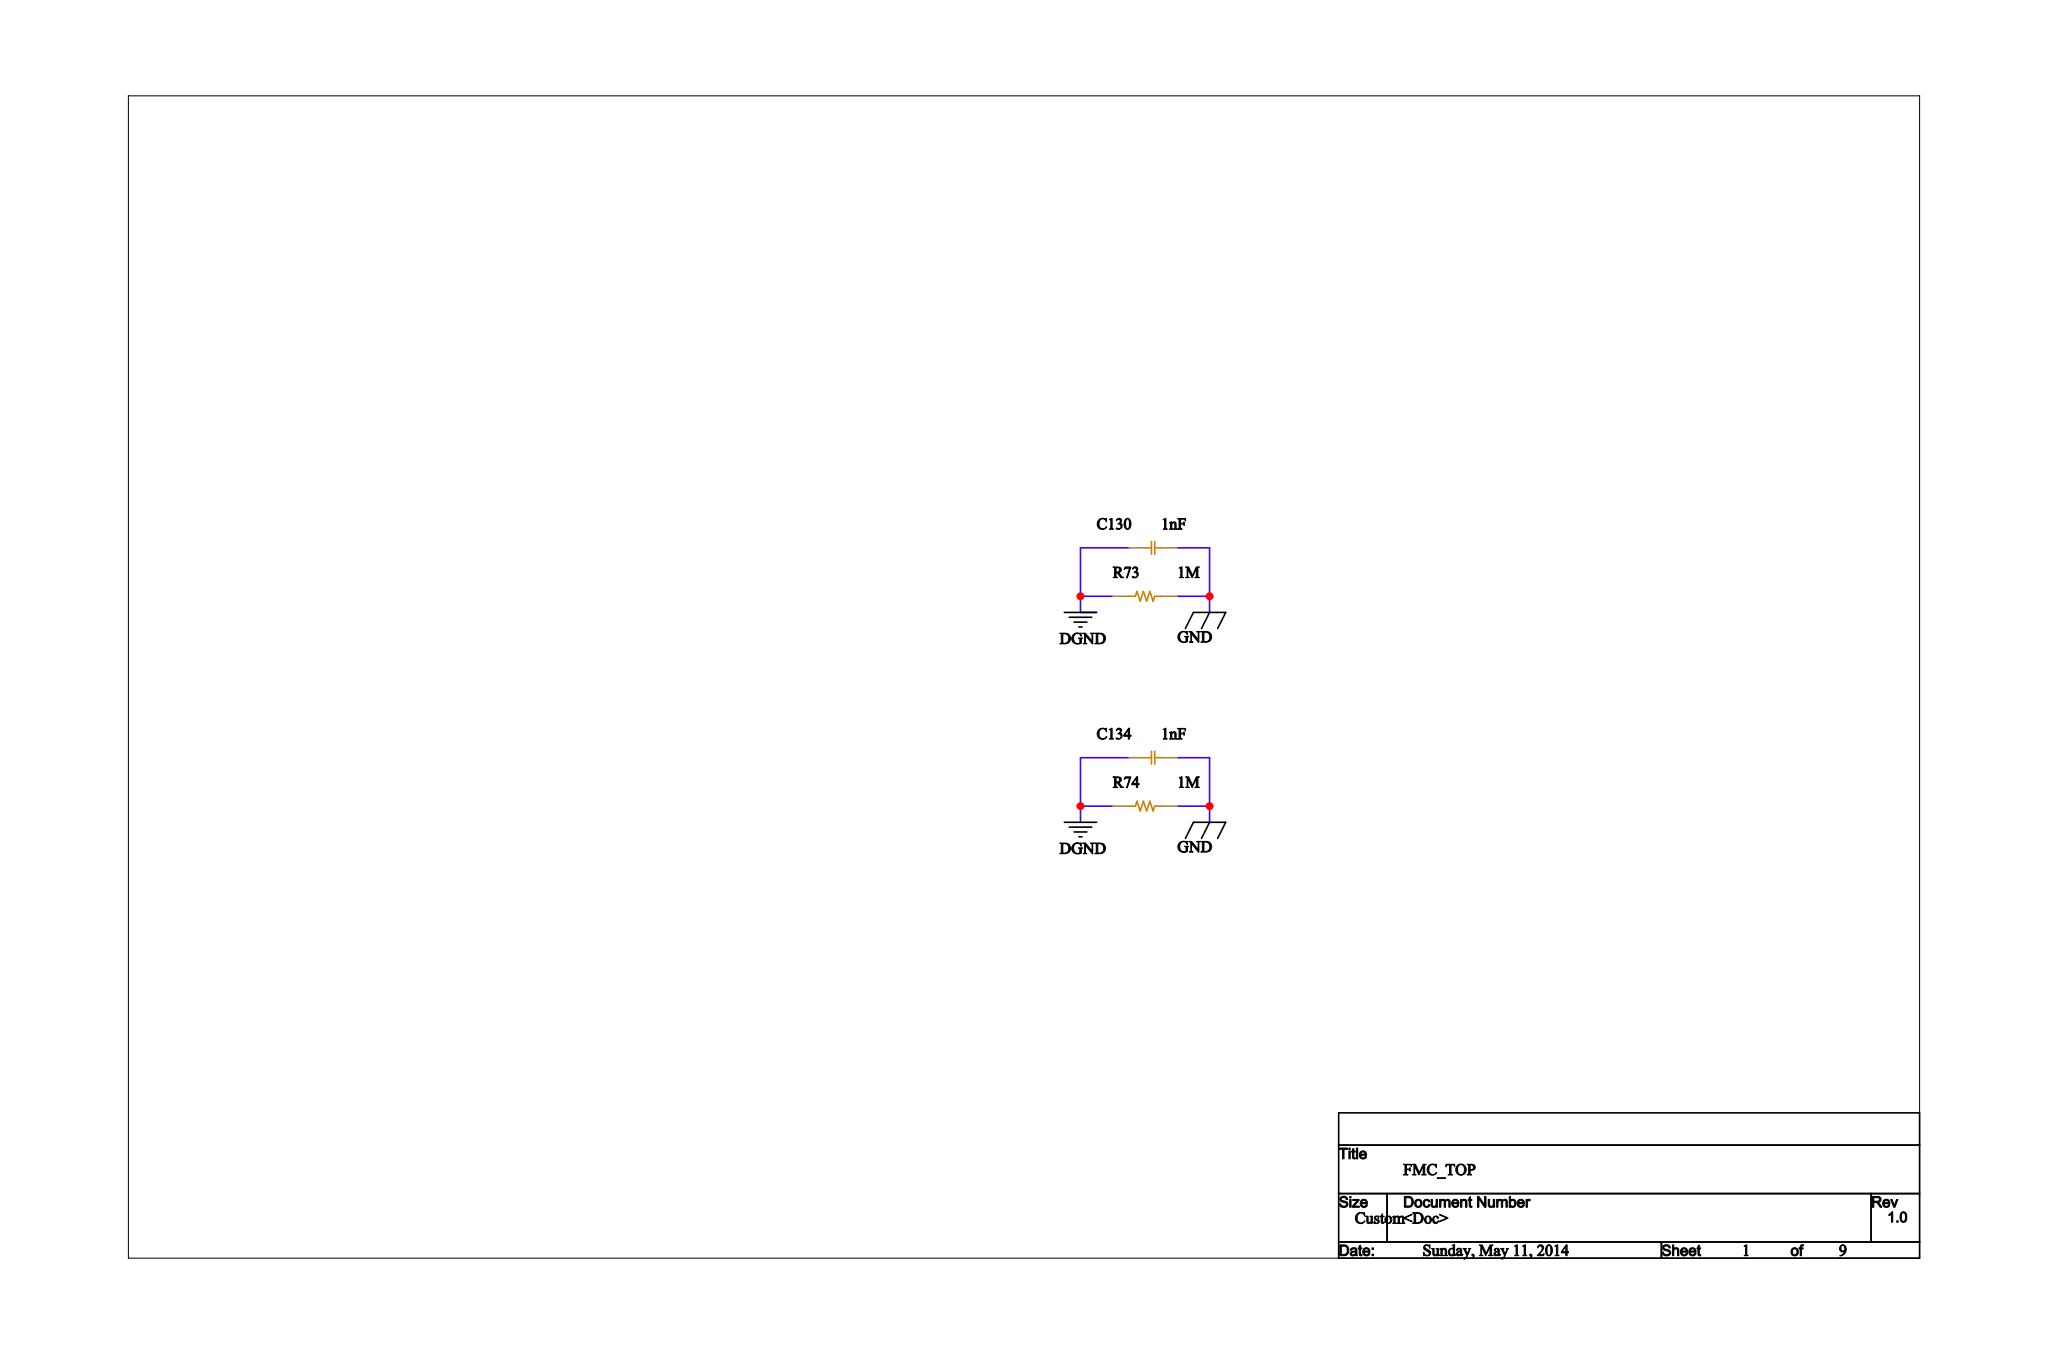Circuit board | Cadence Allegro | 233 parts | 224 nets | one sheet of the schematic
Parts on this sheet (reference | value | footprint):
C130 | 1nF | FPC-1206C
C134 | 1nF | FPC-1206C
R73 | 1M | FPC-0603R
R74 | 1M | FPC-0603R
Nets of these parts (net: part-pin ...):
DGND: C130-1 C134-1 R73-2 R74-2
GND: C130-2 C134-2 R73-1 R74-1